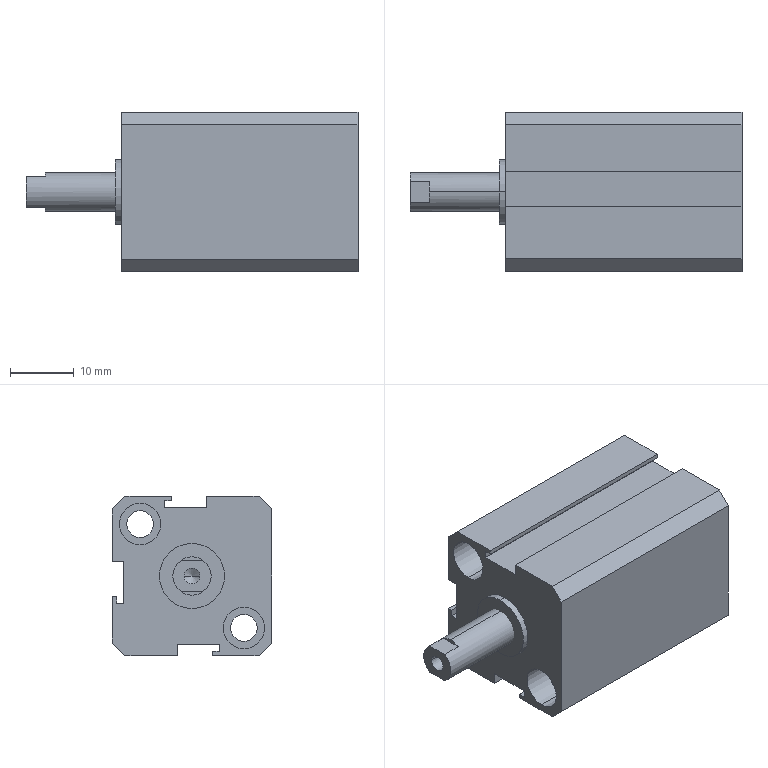Part | STEP file | Cylinder SDA S-12×10 Extend | 2 solids | 59 faces | box 52 x 25 x 25 mm | volume 21189 mm3 | plane 39 | cylinder 18 | cone 2 | commonest cylinder face diameters 6.5 x8 4.2 x4 2.5 x2 6 x2 10.2 x2